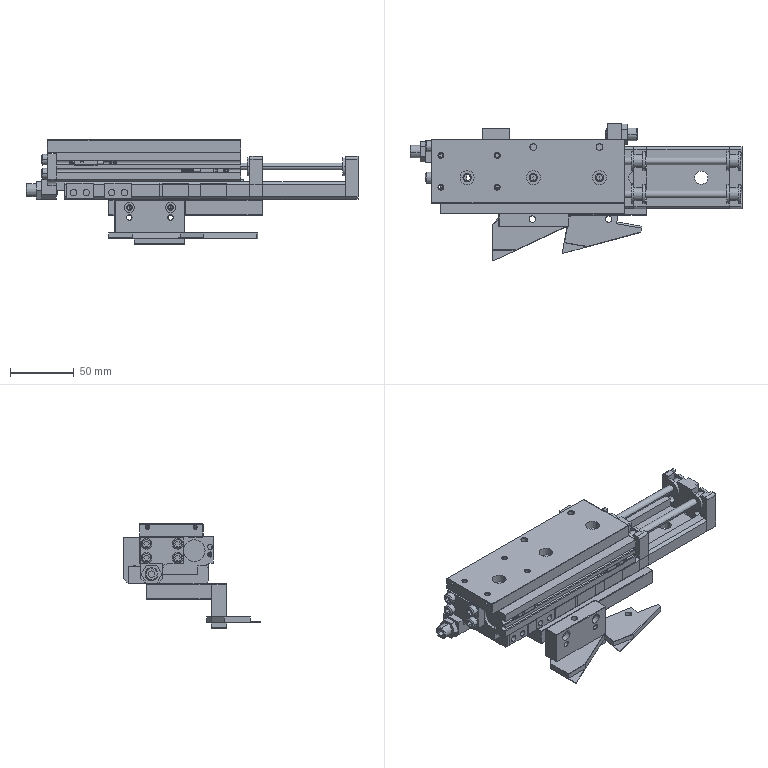Part | NX | 15 solids | 959 faces | box 260.875 x 107.5 x 81.8 mm | volume 539820 mm3 | plane 528 | cylinder 357 | cone 74 | commonest cylinder face diameters 5 x100 2.5 x32 6 x24 9.5 x18 3.3 x16 8.5 x16